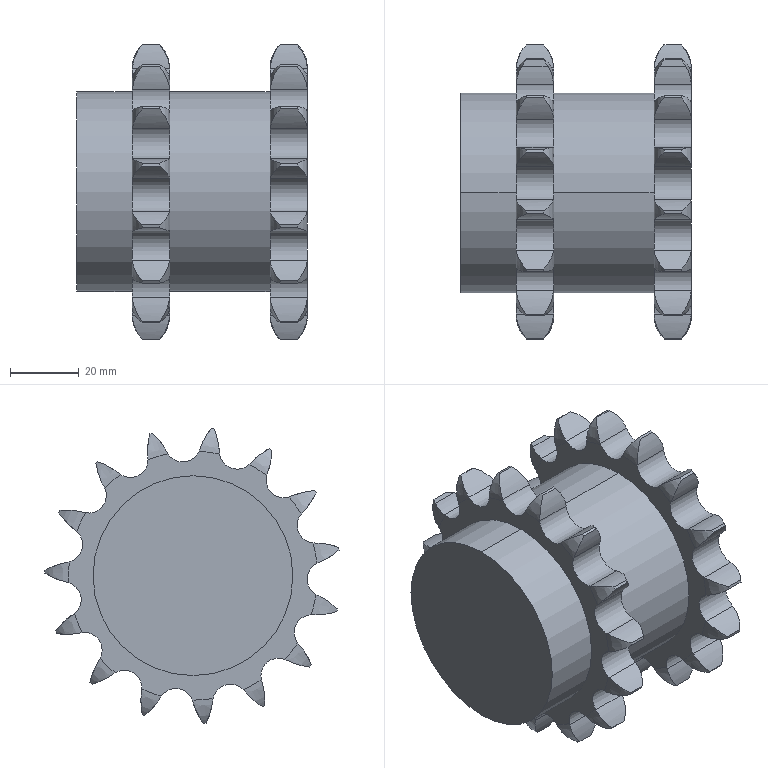Part | SolidWorks | features ICE 8, MoveFace 6, HoleWzd 2, BaseBody 1, Chamfer 1 | 1 solid | 211 faces | box 67.004 x 85.388 x 85.616 mm | volume 208650 mm3 | cylinder 140 | torus 64 | plane 5 | cone 2 | commonest cylinder face diameters 41.452 x62 10.262 x42 86.038 x30 58 x4 10.2 x2